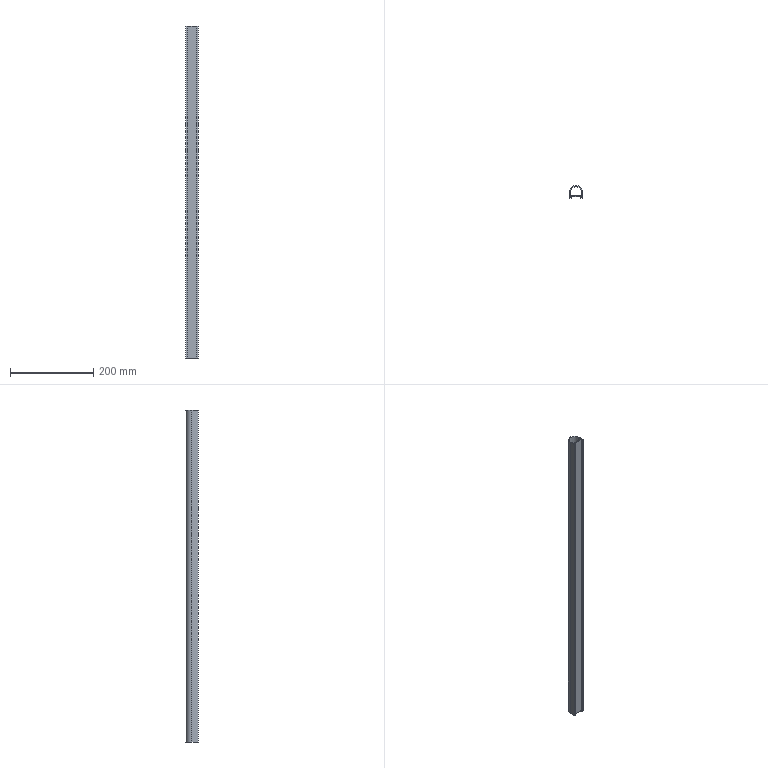Part | SolidWorks | features ICE 2, Extrusion 1 | 1 solid | 18 faces | box 30 x 30 x 800 mm | volume 132921 mm3 | plane 16 | cylinder 2 | commonest cylinder face diameters 27 x1 30 x1
STEP:
#1=CARTESIAN_POINT('',(-55.764,-15.,0.));
#2=VERTEX_POINT('',#1);
#3=CARTESIAN_POINT('',(-51.764,-15.,0.));
#4=VERTEX_POINT('',#3);
#5=CARTESIAN_POINT('',(-25.764,-15.,0.));
#6=DIRECTION('',(1.,0.,0.));
#7=VECTOR('',#6,1000.);
#8=LINE('',#5,#7);
#9=EDGE_CURVE('',#2,#4,#8,.T.);
#10=ORIENTED_EDGE('',*,*,#9,.T.);
#11=CARTESIAN_POINT('',(-51.764,-15.,800.));
#12=VERTEX_POINT('',#11);
#13=CARTESIAN_POINT('',(-51.764,-15.,0.));
#14=DIRECTION('',(0.,0.,1.));
#15=VECTOR('',#14,1000.);
#16=LINE('',#13,#15);
#17=EDGE_CURVE('',#4,#12,#16,.T.);
#18=ORIENTED_EDGE('',*,*,#17,.T.);
#19=CARTESIAN_POINT('',(-55.764,-15.,800.));
#20=VERTEX_POINT('',#19);
#21=CARTESIAN_POINT('',(-25.764,-15.,800.));
#22=DIRECTION('',(1.,0.,0.));
#23=VECTOR('',#22,1000.);
#24=LINE('',#21,#23);
#25=EDGE_CURVE('',#20,#12,#24,.T.);
#26=ORIENTED_EDGE('',*,*,#25,.F.);
#27=CARTESIAN_POINT('',(-55.764,-15.,800.));
#28=DIRECTION('',(0.,0.,-1.));
#29=VECTOR('',#28,1000.);
#30=LINE('',#27,#29);
#31=EDGE_CURVE('',#20,#2,#30,.T.);
#32=ORIENTED_EDGE('',*,*,#31,.T.);
#33=EDGE_LOOP('',(#10,#18,#26,#32));
#34=FACE_OUTER_BOUND('',#33,.T.);
#35=CARTESIAN_POINT('',(-25.764,-15.,800.));
#36=DIRECTION('',(0.,1.,0.));
#37=DIRECTION('',(0.,0.,1.));
#38=AXIS2_PLACEMENT_3D('',#35,#36,#37);
#39=PLANE('',#38);
#40=ADVANCED_FACE('',(#34),#39,.F.);
#41=CARTESIAN_POINT('',(-25.764,0.,0.));
#42=VERTEX_POINT('',#41);
#43=CARTESIAN_POINT('',(-55.764,0.,0.));
#44=VERTEX_POINT('',#43);
#45=CARTESIAN_POINT('',(-40.764,0.,0.));
#46=DIRECTION('',(0.,0.,1.));
#47=DIRECTION('',(1.,0.,0.));
#48=AXIS2_PLACEMENT_3D('',#45,#46,#47);
#49=CIRCLE('',#48,15.);
#50=EDGE_CURVE('',#42,#44,#49,.T.);
#51=ORIENTED_EDGE('',*,*,#50,.T.);
#52=CARTESIAN_POINT('',(-55.764,0.,800.));
#53=VERTEX_POINT('',#52);
#54=CARTESIAN_POINT('',(-55.764,0.,800.));
#55=DIRECTION('',(0.,0.,-1.));
#56=VECTOR('',#55,1000.);
#57=LINE('',#54,#56);
#58=EDGE_CURVE('',#53,#44,#57,.T.);
#59=ORIENTED_EDGE('',*,*,#58,.F.);
#60=CARTESIAN_POINT('',(-25.764,0.,800.));
#61=VERTEX_POINT('',#60);
#62=CARTESIAN_POINT('',(-40.764,0.,800.));
#63=DIRECTION('',(0.,0.,1.));
#64=DIRECTION('',(1.,0.,0.));
#65=AXIS2_PLACEMENT_3D('',#62,#63,#64);
#66=CIRCLE('',#65,15.);
#67=EDGE_CURVE('',#61,#53,#66,.T.);
#68=ORIENTED_EDGE('',*,*,#67,.F.);
#69=CARTESIAN_POINT('',(-25.764,0.,800.));
#70=DIRECTION('',(0.,0.,-1.));
#71=VECTOR('',#70,1000.);
#72=LINE('',#69,#71);
#73=EDGE_CURVE('',#61,#42,#72,.T.);
#74=ORIENTED_EDGE('',*,*,#73,.T.);
#75=EDGE_LOOP('',(#51,#59,#68,#74));
#76=FACE_OUTER_BOUND('',#75,.T.);
#77=CARTESIAN_POINT('',(-40.764,0.,800.));
#78=DIRECTION('',(0.,0.,-1.));
#79=DIRECTION('',(-1.,0.,0.));
#80=AXIS2_PLACEMENT_3D('',#77,#78,#79);
#81=CYLINDRICAL_SURFACE('',#80,15.);
#82=ADVANCED_FACE('',(#76),#81,.T.);
#83=CARTESIAN_POINT('',(-55.764,-15.,0.));
#84=DIRECTION('',(0.,-1.,0.));
#85=VECTOR('',#84,1000.);
#86=LINE('',#83,#85);
#87=EDGE_CURVE('',#44,#2,#86,.T.);
#88=ORIENTED_EDGE('',*,*,#87,.T.);
#89=ORIENTED_EDGE('',*,*,#31,.F.);
#90=CARTESIAN_POINT('',(-55.764,-15.,800.));
#91=DIRECTION('',(0.,-1.,0.));
#92=VECTOR('',#91,1000.);
#93=LINE('',#90,#92);
#94=EDGE_CURVE('',#53,#20,#93,.T.);
#95=ORIENTED_EDGE('',*,*,#94,.F.);
#96=ORIENTED_EDGE('',*,*,#58,.T.);
#97=EDGE_LOOP('',(#88,#89,#95,#96));
#98=FACE_OUTER_BOUND('',#97,.T.);
#99=CARTESIAN_POINT('',(-55.764,-15.,800.));
#100=DIRECTION('',(1.,0.,0.));
#101=DIRECTION('',(0.,0.,-1.));
#102=AXIS2_PLACEMENT_3D('',#99,#100,#101);
#103=PLANE('',#102);
#104=ADVANCED_FACE('',(#98),#103,.F.);
#105=CARTESIAN_POINT('',(-29.764,-15.,800.));
#106=VERTEX_POINT('',#105);
#107=CARTESIAN_POINT('',(-25.764,-15.,800.));
#108=VERTEX_POINT('',#107);
#109=CARTESIAN_POINT('',(-25.764,-15.,800.));
#110=DIRECTION('',(1.,0.,0.));
#111=VECTOR('',#110,1000.);
#112=LINE('',#109,#111);
#113=EDGE_CURVE('',#106,#108,#112,.T.);
#114=ORIENTED_EDGE('',*,*,#113,.F.);
#115=CARTESIAN_POINT('',(-29.764,-15.,0.));
#116=VERTEX_POINT('',#115);
#117=CARTESIAN_POINT('',(-29.764,-15.,0.));
#118=DIRECTION('',(0.,0.,1.));
#119=VECTOR('',#118,1000.);
#120=LINE('',#117,#119);
#121=EDGE_CURVE('',#116,#106,#120,.T.);
#122=ORIENTED_EDGE('',*,*,#121,.F.);
#123=CARTESIAN_POINT('',(-25.764,-15.,0.));
#124=VERTEX_POINT('',#123);
#125=CARTESIAN_POINT('',(-25.764,-15.,0.));
#126=DIRECTION('',(1.,0.,0.));
#127=VECTOR('',#126,1000.);
#128=LINE('',#125,#127);
#129=EDGE_CURVE('',#116,#124,#128,.T.);
#130=ORIENTED_EDGE('',*,*,#129,.T.);
#131=CARTESIAN_POINT('',(-25.764,-15.,800.));
#132=DIRECTION('',(0.,0.,-1.));
#133=VECTOR('',#132,1000.);
#134=LINE('',#131,#133);
#135=EDGE_CURVE('',#108,#124,#134,.T.);
#136=ORIENTED_EDGE('',*,*,#135,.F.);
#137=EDGE_LOOP('',(#114,#122,#130,#136));
#138=FACE_OUTER_BOUND('',#137,.T.);
#139=CARTESIAN_POINT('',(-25.764,-15.,800.));
#140=DIRECTION('',(0.,1.,0.));
#141=DIRECTION('',(0.,0.,1.));
#142=AXIS2_PLACEMENT_3D('',#139,#140,#141);
#143=PLANE('',#142);
#144=ADVANCED_FACE('',(#138),#143,.F.);
#145=CARTESIAN_POINT('',(-25.764,0.,0.));
#146=DIRECTION('',(0.,1.,0.));
#147=VECTOR('',#146,1000.);
#148=LINE('',#145,#147);
#149=EDGE_CURVE('',#124,#42,#148,.T.);
#150=ORIENTED_EDGE('',*,*,#149,.T.);
#151=ORIENTED_EDGE('',*,*,#73,.F.);
#152=CARTESIAN_POINT('',(-25.764,0.,800.));
#153=DIRECTION('',(0.,1.,0.));
#154=VECTOR('',#153,1000.);
#155=LINE('',#152,#154);
#156=EDGE_CURVE('',#108,#61,#155,.T.);
#157=ORIENTED_EDGE('',*,*,#156,.F.);
#158=ORIENTED_EDGE('',*,*,#135,.T.);
#159=EDGE_LOOP('',(#150,#151,#157,#158));
#160=FACE_OUTER_BOUND('',#159,.T.);
#161=CARTESIAN_POINT('',(-25.764,0.,800.));
#162=DIRECTION('',(-1.,0.,0.));
#163=DIRECTION('',(0.,0.,1.));
#164=AXIS2_PLACEMENT_3D('',#161,#162,#163);
#165=PLANE('',#164);
#166=ADVANCED_FACE('',(#160),#165,.F.);
#167=CARTESIAN_POINT('',(-51.764,-13.5,800.));
#168=VERTEX_POINT('',#167);
#169=CARTESIAN_POINT('',(-51.764,-15.,800.));
#170=DIRECTION('',(0.,-1.,0.));
#171=VECTOR('',#170,1000.);
#172=LINE('',#169,#171);
#173=EDGE_CURVE('',#168,#12,#172,.T.);
#174=ORIENTED_EDGE('',*,*,#173,.F.);
#175=CARTESIAN_POINT('',(-53.264,-13.5,800.));
#176=VERTEX_POINT('',#175);
#177=CARTESIAN_POINT('',(-51.764,-13.5,800.));
#178=DIRECTION('',(1.,0.,0.));
#179=VECTOR('',#178,1000.);
#180=LINE('',#177,#179);
#181=EDGE_CURVE('',#176,#168,#180,.T.);
#182=ORIENTED_EDGE('',*,*,#181,.F.);
#183=CARTESIAN_POINT('',(-53.264,-10.5,800.));
#184=VERTEX_POINT('',#183);
#185=CARTESIAN_POINT('',(-53.264,-13.5,800.));
#186=DIRECTION('',(0.,-1.,0.));
#187=VECTOR('',#186,1000.);
#188=LINE('',#185,#187);
#189=EDGE_CURVE('',#184,#176,#188,.T.);
#190=ORIENTED_EDGE('',*,*,#189,.F.);
#191=CARTESIAN_POINT('',(-28.264,-10.5,800.));
#192=VERTEX_POINT('',#191);
#193=CARTESIAN_POINT('',(-28.264,-10.5,800.));
#194=DIRECTION('',(-1.,0.,0.));
#195=VECTOR('',#194,1000.);
#196=LINE('',#193,#195);
#197=EDGE_CURVE('',#192,#184,#196,.T.);
#198=ORIENTED_EDGE('',*,*,#197,.F.);
#199=CARTESIAN_POINT('',(-28.264,-13.5,800.));
#200=VERTEX_POINT('',#199);
#201=CARTESIAN_POINT('',(-28.264,-13.5,800.));
#202=DIRECTION('',(0.,1.,0.));
#203=VECTOR('',#202,1000.);
#204=LINE('',#201,#203);
#205=EDGE_CURVE('',#200,#192,#204,.T.);
#206=ORIENTED_EDGE('',*,*,#205,.F.);
#207=CARTESIAN_POINT('',(-29.764,-13.5,800.));
#208=VERTEX_POINT('',#207);
#209=CARTESIAN_POINT('',(-29.764,-13.5,800.));
#210=DIRECTION('',(1.,0.,0.));
#211=VECTOR('',#210,1000.);
#212=LINE('',#209,#211);
#213=EDGE_CURVE('',#208,#200,#212,.T.);
#214=ORIENTED_EDGE('',*,*,#213,.F.);
#215=CARTESIAN_POINT('',(-29.764,-15.,800.));
#216=DIRECTION('',(0.,1.,0.));
#217=VECTOR('',#216,1000.);
#218=LINE('',#215,#217);
#219=EDGE_CURVE('',#106,#208,#218,.T.);
#220=ORIENTED_EDGE('',*,*,#219,.F.);
#221=ORIENTED_EDGE('',*,*,#113,.T.);
#222=ORIENTED_EDGE('',*,*,#156,.T.);
#223=ORIENTED_EDGE('',*,*,#67,.T.);
#224=ORIENTED_EDGE('',*,*,#94,.T.);
#225=ORIENTED_EDGE('',*,*,#25,.T.);
#226=EDGE_LOOP('',(#174,#182,#190,#198,#206,#214,#220,#221,#222,#223,#224,#225));
#227=FACE_OUTER_BOUND('',#226,.T.);
#228=CARTESIAN_POINT('',(-27.264,0.,800.));
#229=VERTEX_POINT('',#228);
#230=CARTESIAN_POINT('',(-54.264,0.,800.));
#231=VERTEX_POINT('',#230);
#232=CARTESIAN_POINT('',(-40.764,0.,800.));
#233=DIRECTION('',(0.,0.,1.));
#234=DIRECTION('',(1.,0.,0.));
#235=AXIS2_PLACEMENT_3D('',#232,#233,#234);
#236=CIRCLE('',#235,13.5);
#237=EDGE_CURVE('',#229,#231,#236,.T.);
#238=ORIENTED_EDGE('',*,*,#237,.F.);
#239=CARTESIAN_POINT('',(-27.264,-9.,800.));
#240=VERTEX_POINT('',#239);
#241=CARTESIAN_POINT('',(-27.264,0.,800.));
#242=DIRECTION('',(0.,1.,0.));
#243=VECTOR('',#242,1000.);
#244=LINE('',#241,#243);
#245=EDGE_CURVE('',#240,#229,#244,.T.);
#246=ORIENTED_EDGE('',*,*,#245,.F.);
#247=CARTESIAN_POINT('',(-54.264,-9.,800.));
#248=VERTEX_POINT('',#247);
#249=CARTESIAN_POINT('',(-54.264,-9.,800.));
#250=DIRECTION('',(1.,0.,0.));
#251=VECTOR('',#250,1000.);
#252=LINE('',#249,#251);
#253=EDGE_CURVE('',#248,#240,#252,.T.);
#254=ORIENTED_EDGE('',*,*,#253,.F.);
#255=CARTESIAN_POINT('',(-54.264,0.,800.));
#256=DIRECTION('',(0.,-1.,0.));
#257=VECTOR('',#256,1000.);
#258=LINE('',#255,#257);
#259=EDGE_CURVE('',#231,#248,#258,.T.);
#260=ORIENTED_EDGE('',*,*,#259,.F.);
#261=EDGE_LOOP('',(#238,#246,#254,#260));
#262=FACE_BOUND('',#261,.T.);
#263=CARTESIAN_POINT('',(-40.764,0.,800.));
#264=DIRECTION('',(0.,0.,1.));
#265=DIRECTION('',(1.,0.,0.));
#266=AXIS2_PLACEMENT_3D('',#263,#264,#265);
#267=PLANE('',#266);
#268=ADVANCED_FACE('',(#227,#262),#267,.T.);
#269=CARTESIAN_POINT('',(-27.264,-9.,0.));
#270=VERTEX_POINT('',#269);
#271=CARTESIAN_POINT('',(-27.264,0.,0.));
#272=VERTEX_POINT('',#271);
#273=CARTESIAN_POINT('',(-27.264,0.,0.));
#274=DIRECTION('',(0.,1.,0.));
#275=VECTOR('',#274,1000.);
#276=LINE('',#273,#275);
#277=EDGE_CURVE('',#270,#272,#276,.T.);
#278=ORIENTED_EDGE('',*,*,#277,.T.);
#279=CARTESIAN_POINT('',(-54.264,0.,0.));
#280=VERTEX_POINT('',#279);
#281=CARTESIAN_POINT('',(-40.764,0.,0.));
#282=DIRECTION('',(0.,0.,1.));
#283=DIRECTION('',(1.,0.,0.));
#284=AXIS2_PLACEMENT_3D('',#281,#282,#283);
#285=CIRCLE('',#284,13.5);
#286=EDGE_CURVE('',#272,#280,#285,.T.);
#287=ORIENTED_EDGE('',*,*,#286,.T.);
#288=CARTESIAN_POINT('',(-54.264,-9.,0.));
#289=VERTEX_POINT('',#288);
#290=CARTESIAN_POINT('',(-54.264,0.,0.));
#291=DIRECTION('',(0.,-1.,0.));
#292=VECTOR('',#291,1000.);
#293=LINE('',#290,#292);
#294=EDGE_CURVE('',#280,#289,#293,.T.);
#295=ORIENTED_EDGE('',*,*,#294,.T.);
#296=CARTESIAN_POINT('',(-54.264,-9.,0.));
#297=DIRECTION('',(1.,0.,0.));
#298=VECTOR('',#297,1000.);
#299=LINE('',#296,#298);
#300=EDGE_CURVE('',#289,#270,#299,.T.);
#301=ORIENTED_EDGE('',*,*,#300,.T.);
#302=EDGE_LOOP('',(#278,#287,#295,#301));
#303=FACE_BOUND('',#302,.T.);
#304=CARTESIAN_POINT('',(-53.264,-13.5,0.));
#305=VERTEX_POINT('',#304);
#306=CARTESIAN_POINT('',(-51.764,-13.5,0.));
#307=VERTEX_POINT('',#306);
#308=CARTESIAN_POINT('',(-51.764,-13.5,0.));
#309=DIRECTION('',(1.,0.,0.));
#310=VECTOR('',#309,1000.);
#311=LINE('',#308,#310);
#312=EDGE_CURVE('',#305,#307,#311,.T.);
#313=ORIENTED_EDGE('',*,*,#312,.T.);
#314=CARTESIAN_POINT('',(-51.764,-15.,0.));
#315=DIRECTION('',(0.,-1.,0.));
#316=VECTOR('',#315,1000.);
#317=LINE('',#314,#316);
#318=EDGE_CURVE('',#307,#4,#317,.T.);
#319=ORIENTED_EDGE('',*,*,#318,.T.);
#320=ORIENTED_EDGE('',*,*,#9,.F.);
#321=ORIENTED_EDGE('',*,*,#87,.F.);
#322=ORIENTED_EDGE('',*,*,#50,.F.);
#323=ORIENTED_EDGE('',*,*,#149,.F.);
#324=ORIENTED_EDGE('',*,*,#129,.F.);
#325=CARTESIAN_POINT('',(-29.764,-13.5,0.));
#326=VERTEX_POINT('',#325);
#327=CARTESIAN_POINT('',(-29.764,-15.,0.));
#328=DIRECTION('',(0.,1.,0.));
#329=VECTOR('',#328,1000.);
#330=LINE('',#327,#329);
#331=EDGE_CURVE('',#116,#326,#330,.T.);
#332=ORIENTED_EDGE('',*,*,#331,.T.);
#333=CARTESIAN_POINT('',(-28.264,-13.5,0.));
#334=VERTEX_POINT('',#333);
#335=CARTESIAN_POINT('',(-29.764,-13.5,0.));
#336=DIRECTION('',(1.,0.,0.));
#337=VECTOR('',#336,1000.);
#338=LINE('',#335,#337);
#339=EDGE_CURVE('',#326,#334,#338,.T.);
#340=ORIENTED_EDGE('',*,*,#339,.T.);
#341=CARTESIAN_POINT('',(-28.264,-10.5,0.));
#342=VERTEX_POINT('',#341);
#343=CARTESIAN_POINT('',(-28.264,-13.5,0.));
#344=DIRECTION('',(0.,1.,0.));
#345=VECTOR('',#344,1000.);
#346=LINE('',#343,#345);
#347=EDGE_CURVE('',#334,#342,#346,.T.);
#348=ORIENTED_EDGE('',*,*,#347,.T.);
#349=CARTESIAN_POINT('',(-53.264,-10.5,0.));
#350=VERTEX_POINT('',#349);
#351=CARTESIAN_POINT('',(-28.264,-10.5,0.));
#352=DIRECTION('',(-1.,0.,0.));
#353=VECTOR('',#352,1000.);
#354=LINE('',#351,#353);
#355=EDGE_CURVE('',#342,#350,#354,.T.);
#356=ORIENTED_EDGE('',*,*,#355,.T.);
#357=CARTESIAN_POINT('',(-53.264,-13.5,0.));
#358=DIRECTION('',(0.,-1.,0.));
#359=VECTOR('',#358,1000.);
#360=LINE('',#357,#359);
#361=EDGE_CURVE('',#350,#305,#360,.T.);
#362=ORIENTED_EDGE('',*,*,#361,.T.);
#363=EDGE_LOOP('',(#313,#319,#320,#321,#322,#323,#324,#332,#340,#348,#356,#362));
#364=FACE_OUTER_BOUND('',#363,.T.);
#365=CARTESIAN_POINT('',(-40.764,0.,0.));
#366=DIRECTION('',(0.,0.,1.));
#367=DIRECTION('',(1.,0.,0.));
#368=AXIS2_PLACEMENT_3D('',#365,#366,#367);
#369=PLANE('',#368);
#370=ADVANCED_FACE('',(#303,#364),#369,.F.);
#371=ORIENTED_EDGE('',*,*,#237,.T.);
#372=CARTESIAN_POINT('',(-54.264,0.,0.));
#373=DIRECTION('',(0.,0.,1.));
#374=VECTOR('',#373,1000.);
#375=LINE('',#372,#374);
#376=EDGE_CURVE('',#280,#231,#375,.T.);
#377=ORIENTED_EDGE('',*,*,#376,.F.);
#378=ORIENTED_EDGE('',*,*,#286,.F.);
#379=CARTESIAN_POINT('',(-27.264,0.,0.));
#380=DIRECTION('',(0.,0.,1.));
#381=VECTOR('',#380,1000.);
#382=LINE('',#379,#381);
#383=EDGE_CURVE('',#272,#229,#382,.T.);
#384=ORIENTED_EDGE('',*,*,#383,.T.);
#385=EDGE_LOOP('',(#371,#377,#378,#384));
#386=FACE_OUTER_BOUND('',#385,.T.);
#387=CARTESIAN_POINT('',(-40.764,0.,0.));
#388=DIRECTION('',(0.,0.,1.));
#389=DIRECTION('',(1.,0.,0.));
#390=AXIS2_PLACEMENT_3D('',#387,#388,#389);
#391=CYLINDRICAL_SURFACE('',#390,13.5);
#392=ADVANCED_FACE('',(#386),#391,.F.);
#393=ORIENTED_EDGE('',*,*,#245,.T.);
#394=ORIENTED_EDGE('',*,*,#383,.F.);
#395=ORIENTED_EDGE('',*,*,#277,.F.);
#396=CARTESIAN_POINT('',(-27.264,-9.,0.));
#397=DIRECTION('',(0.,0.,1.));
#398=VECTOR('',#397,1000.);
#399=LINE('',#396,#398);
#400=EDGE_CURVE('',#270,#240,#399,.T.);
#401=ORIENTED_EDGE('',*,*,#400,.T.);
#402=EDGE_LOOP('',(#393,#394,#395,#401));
#403=FACE_OUTER_BOUND('',#402,.T.);
#404=CARTESIAN_POINT('',(-27.264,0.,0.));
#405=DIRECTION('',(1.,0.,0.));
#406=DIRECTION('',(0.,0.,-1.));
#407=AXIS2_PLACEMENT_3D('',#404,#405,#406);
#408=PLANE('',#407);
#409=ADVANCED_FACE('',(#403),#408,.F.);
#410=ORIENTED_EDGE('',*,*,#253,.T.);
#411=ORIENTED_EDGE('',*,*,#400,.F.);
#412=ORIENTED_EDGE('',*,*,#300,.F.);
#413=CARTESIAN_POINT('',(-54.264,-9.,0.));
#414=DIRECTION('',(0.,0.,1.));
#415=VECTOR('',#414,1000.);
#416=LINE('',#413,#415);
#417=EDGE_CURVE('',#289,#248,#416,.T.);
#418=ORIENTED_EDGE('',*,*,#417,.T.);
#419=EDGE_LOOP('',(#410,#411,#412,#418));
#420=FACE_OUTER_BOUND('',#419,.T.);
#421=CARTESIAN_POINT('',(-54.264,-9.,0.));
#422=DIRECTION('',(0.,-1.,0.));
#423=DIRECTION('',(0.,0.,-1.));
#424=AXIS2_PLACEMENT_3D('',#421,#422,#423);
#425=PLANE('',#424);
#426=ADVANCED_FACE('',(#420),#425,.F.);
#427=ORIENTED_EDGE('',*,*,#259,.T.);
#428=ORIENTED_EDGE('',*,*,#417,.F.);
#429=ORIENTED_EDGE('',*,*,#294,.F.);
#430=ORIENTED_EDGE('',*,*,#376,.T.);
#431=EDGE_LOOP('',(#427,#428,#429,#430));
#432=FACE_OUTER_BOUND('',#431,.T.);
#433=CARTESIAN_POINT('',(-54.264,0.,0.));
#434=DIRECTION('',(-1.,0.,0.));
#435=DIRECTION('',(0.,0.,1.));
#436=AXIS2_PLACEMENT_3D('',#433,#434,#435);
#437=PLANE('',#436);
#438=ADVANCED_FACE('',(#432),#437,.F.);
#439=ORIENTED_EDGE('',*,*,#173,.T.);
#440=ORIENTED_EDGE('',*,*,#17,.F.);
#441=ORIENTED_EDGE('',*,*,#318,.F.);
#442=CARTESIAN_POINT('',(-51.764,-13.5,0.));
#443=DIRECTION('',(0.,0.,1.));
#444=VECTOR('',#443,1000.);
#445=LINE('',#442,#444);
#446=EDGE_CURVE('',#307,#168,#445,.T.);
#447=ORIENTED_EDGE('',*,*,#446,.T.);
#448=EDGE_LOOP('',(#439,#440,#441,#447));
#449=FACE_OUTER_BOUND('',#448,.T.);
#450=CARTESIAN_POINT('',(-51.764,-15.,0.));
#451=DIRECTION('',(-1.,0.,0.));
#452=DIRECTION('',(0.,0.,1.));
#453=AXIS2_PLACEMENT_3D('',#450,#451,#452);
#454=PLANE('',#453);
#455=ADVANCED_FACE('',(#449),#454,.F.);
#456=ORIENTED_EDGE('',*,*,#181,.T.);
#457=ORIENTED_EDGE('',*,*,#446,.F.);
#458=ORIENTED_EDGE('',*,*,#312,.F.);
#459=CARTESIAN_POINT('',(-53.264,-13.5,0.));
#460=DIRECTION('',(0.,0.,1.));
#461=VECTOR('',#460,1000.);
#462=LINE('',#459,#461);
#463=EDGE_CURVE('',#305,#176,#462,.T.);
#464=ORIENTED_EDGE('',*,*,#463,.T.);
#465=EDGE_LOOP('',(#456,#457,#458,#464));
#466=FACE_OUTER_BOUND('',#465,.T.);
#467=CARTESIAN_POINT('',(-51.764,-13.5,0.));
#468=DIRECTION('',(0.,-1.,0.));
#469=DIRECTION('',(0.,0.,-1.));
#470=AXIS2_PLACEMENT_3D('',#467,#468,#469);
#471=PLANE('',#470);
#472=ADVANCED_FACE('',(#466),#471,.F.);
#473=ORIENTED_EDGE('',*,*,#189,.T.);
#474=ORIENTED_EDGE('',*,*,#463,.F.);
#475=ORIENTED_EDGE('',*,*,#361,.F.);
#476=CARTESIAN_POINT('',(-53.264,-10.5,0.));
#477=DIRECTION('',(0.,0.,1.));
#478=VECTOR('',#477,1000.);
#479=LINE('',#476,#478);
#480=EDGE_CURVE('',#350,#184,#479,.T.);
#481=ORIENTED_EDGE('',*,*,#480,.T.);
#482=EDGE_LOOP('',(#473,#474,#475,#481));
#483=FACE_OUTER_BOUND('',#482,.T.);
#484=CARTESIAN_POINT('',(-53.264,-13.5,0.));
#485=DIRECTION('',(-1.,0.,0.));
#486=DIRECTION('',(0.,0.,1.));
#487=AXIS2_PLACEMENT_3D('',#484,#485,#486);
#488=PLANE('',#487);
#489=ADVANCED_FACE('',(#483),#488,.F.);
#490=ORIENTED_EDGE('',*,*,#197,.T.);
#491=ORIENTED_EDGE('',*,*,#480,.F.);
#492=ORIENTED_EDGE('',*,*,#355,.F.);
#493=CARTESIAN_POINT('',(-28.264,-10.5,0.));
#494=DIRECTION('',(0.,0.,1.));
#495=VECTOR('',#494,1000.);
#496=LINE('',#493,#495);
#497=EDGE_CURVE('',#342,#192,#496,.T.);
#498=ORIENTED_EDGE('',*,*,#497,.T.);
#499=EDGE_LOOP('',(#490,#491,#492,#498));
#500=FACE_OUTER_BOUND('',#499,.T.);
#501=CARTESIAN_POINT('',(-28.264,-10.5,0.));
#502=DIRECTION('',(0.,1.,0.));
#503=DIRECTION('',(0.,0.,1.));
#504=AXIS2_PLACEMENT_3D('',#501,#502,#503);
#505=PLANE('',#504);
#506=ADVANCED_FACE('',(#500),#505,.F.);
#507=ORIENTED_EDGE('',*,*,#205,.T.);
#508=ORIENTED_EDGE('',*,*,#497,.F.);
#509=ORIENTED_EDGE('',*,*,#347,.F.);
#510=CARTESIAN_POINT('',(-28.264,-13.5,0.));
#511=DIRECTION('',(0.,0.,1.));
#512=VECTOR('',#511,1000.);
#513=LINE('',#510,#512);
#514=EDGE_CURVE('',#334,#200,#513,.T.);
#515=ORIENTED_EDGE('',*,*,#514,.T.);
#516=EDGE_LOOP('',(#507,#508,#509,#515));
#517=FACE_OUTER_BOUND('',#516,.T.);
#518=CARTESIAN_POINT('',(-28.264,-13.5,0.));
#519=DIRECTION('',(1.,0.,0.));
#520=DIRECTION('',(0.,0.,-1.));
#521=AXIS2_PLACEMENT_3D('',#518,#519,#520);
#522=PLANE('',#521);
#523=ADVANCED_FACE('',(#517),#522,.F.);
#524=ORIENTED_EDGE('',*,*,#213,.T.);
#525=ORIENTED_EDGE('',*,*,#514,.F.);
#526=ORIENTED_EDGE('',*,*,#339,.F.);
#527=CARTESIAN_POINT('',(-29.764,-13.5,0.));
#528=DIRECTION('',(0.,0.,1.));
#529=VECTOR('',#528,1000.);
#530=LINE('',#527,#529);
#531=EDGE_CURVE('',#326,#208,#530,.T.);
#532=ORIENTED_EDGE('',*,*,#531,.T.);
#533=EDGE_LOOP('',(#524,#525,#526,#532));
#534=FACE_OUTER_BOUND('',#533,.T.);
#535=CARTESIAN_POINT('',(-29.764,-13.5,0.));
#536=DIRECTION('',(0.,-1.,0.));
#537=DIRECTION('',(0.,0.,-1.));
#538=AXIS2_PLACEMENT_3D('',#535,#536,#537);
#539=PLANE('',#538);
#540=ADVANCED_FACE('',(#534),#539,.F.);
#541=ORIENTED_EDGE('',*,*,#219,.T.);
#542=ORIENTED_EDGE('',*,*,#531,.F.);
#543=ORIENTED_EDGE('',*,*,#331,.F.);
#544=ORIENTED_EDGE('',*,*,#121,.T.);
#545=EDGE_LOOP('',(#541,#542,#543,#544));
#546=FACE_OUTER_BOUND('',#545,.T.);
#547=CARTESIAN_POINT('',(-29.764,-15.,0.));
#548=DIRECTION('',(1.,0.,0.));
#549=DIRECTION('',(0.,0.,-1.));
#550=AXIS2_PLACEMENT_3D('',#547,#548,#549);
#551=PLANE('',#550);
#552=ADVANCED_FACE('',(#546),#551,.F.);
#553=CLOSED_SHELL('',(#40,#82,#104,#144,#166,#268,#370,#392,#409,#426,#438,#455,#472,#489,#506,#523,#540,#552));
#554=MANIFOLD_SOLID_BREP('',#553);
#555=CARTESIAN_POINT('',(0.,0.,0.));
#556=DIRECTION('',(0.,0.,1.));
#557=DIRECTION('',(1.,0.,0.));
#558=AXIS2_PLACEMENT_3D('',#555,#556,#557);
#559=(LENGTH_UNIT()NAMED_UNIT(*)SI_UNIT(.MILLI.,.METRE.));
#560=UNCERTAINTY_MEASURE_WITH_UNIT(LENGTH_MEASURE(0.00001),#559,'','');
#561=(NAMED_UNIT(*)PLANE_ANGLE_UNIT()SI_UNIT($,.RADIAN.));
#562=(NAMED_UNIT(*)SI_UNIT($,.STERADIAN.)SOLID_ANGLE_UNIT());
#563=(GEOMETRIC_REPRESENTATION_CONTEXT(3)GLOBAL_UNCERTAINTY_ASSIGNED_CONTEXT((#560))GLOBAL_UNIT_ASSIGNED_CONTEXT((#559,#561,#562))REPRESENTATION_CONTEXT('',''));
#564=ADVANCED_BREP_SHAPE_REPRESENTATION('',(#554,#558),#563);